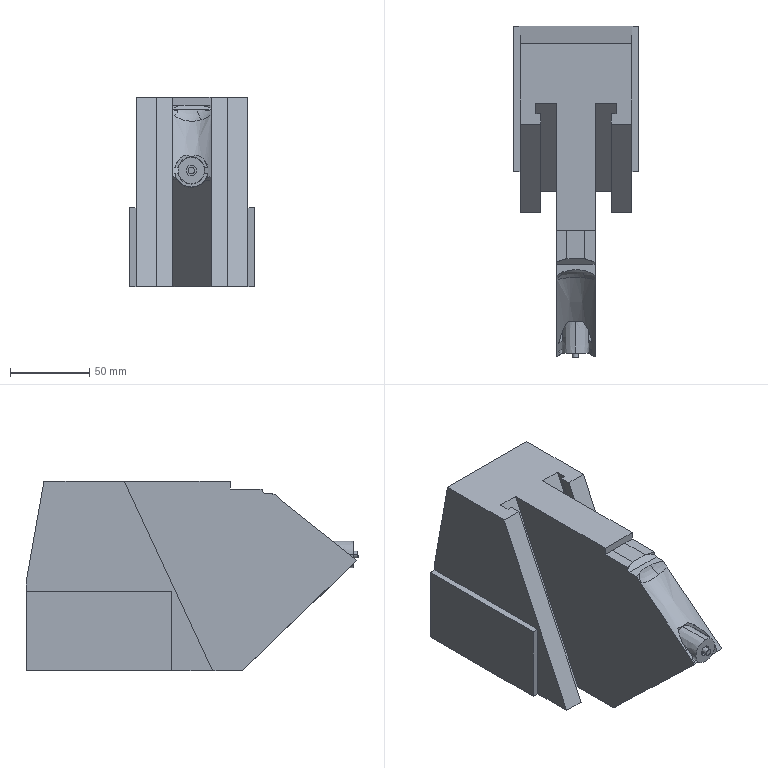Part | Creo | 1 solid | 60 faces | box 78.786 x 209.848 x 119.606 mm | volume 973872 mm3 | plane 39 | cone 9 | cylinder 8 | spline 3 | other 1 | commonest cylinder face diameters 4.02 x2 6.533 x2 58.878 x1 609.334 x1 813.946 x1 44300 x1